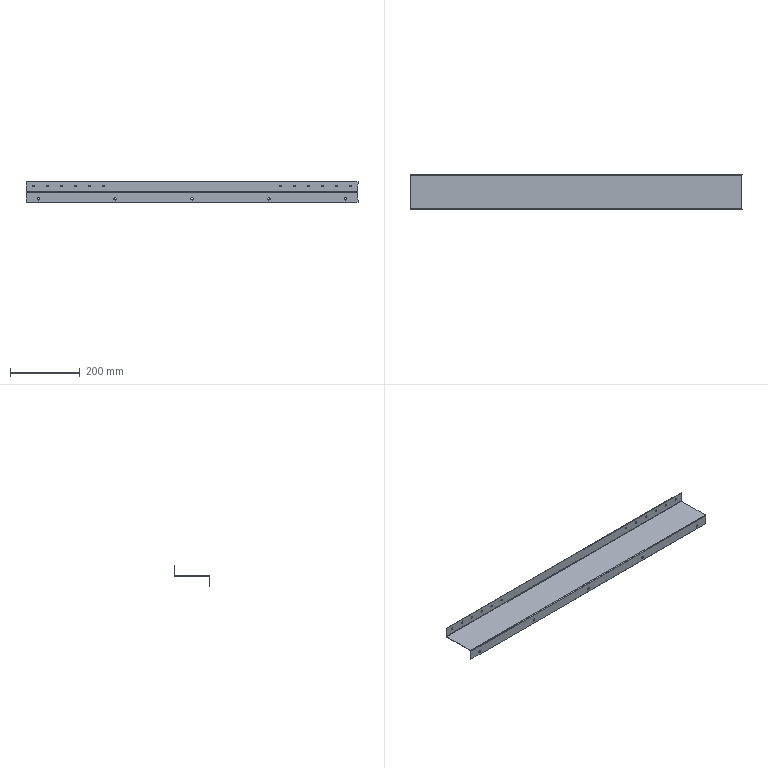Part | SolidWorks | features EdgeFlange 2, HoleWzd 2, FlatPattern 1, LPattern 1, SMBaseFlange 1, SheetMetal 1 | 1 solid | 56 faces | box 950 x 100 x 58.8 mm | volume 177585 mm3 | cylinder 38 | plane 18 | commonest cylinder face diameters 5 x24 7 x10 2 x2 4.4 x2